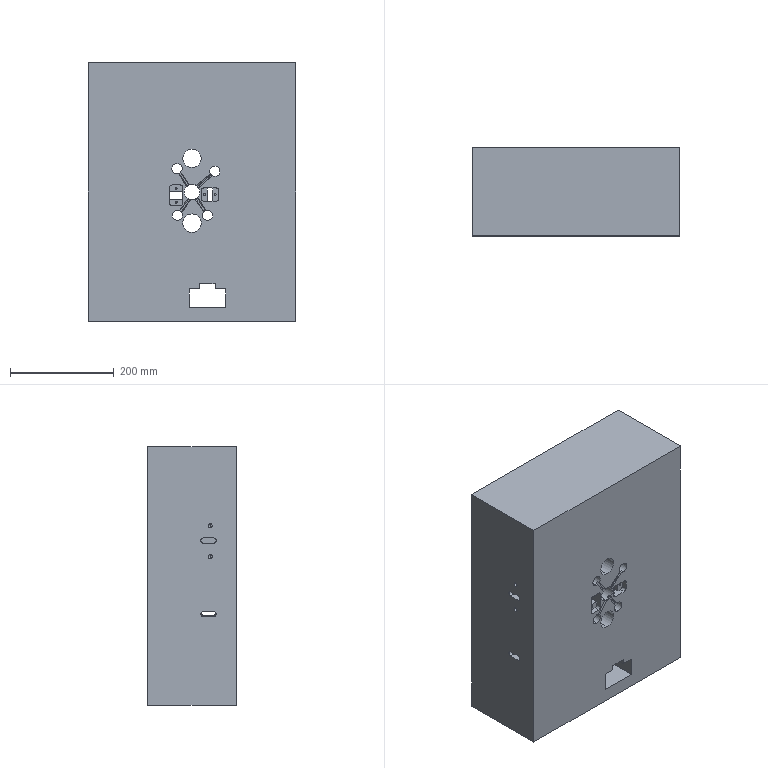Part | STEP file | 1 solid | 282 faces | box 400 x 170 x 500 mm | volume 24400760 mm3 | plane 138 | cylinder 132 | cone 12 | commonest cylinder face diameters 10 x42 8 x16 11 x16 26 x14 16 x12 4 x8